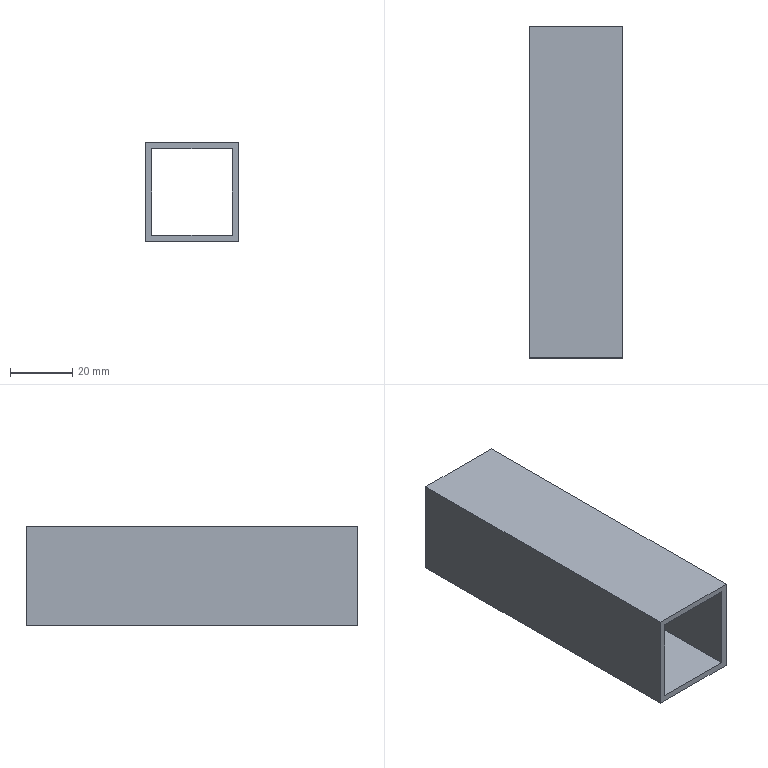Part | NX | features solid 2 | 1 solid | 10 faces | box 30 x 107 x 32 mm | volume 24824 mm3 | plane 10
STEP:
#1=CARTESIAN_POINT('',(475.,468.,-63.));
#2=VERTEX_POINT('',#1);
#3=CARTESIAN_POINT('',(445.,468.,-63.));
#4=VERTEX_POINT('',#3);
#5=CARTESIAN_POINT('',(475.,468.,-63.));
#6=DIRECTION('',(-1.,0.,0.));
#7=VECTOR('',#6,1000.);
#8=LINE('',#5,#7);
#9=EDGE_CURVE('',#2,#4,#8,.T.);
#10=ORIENTED_EDGE('',*,*,#9,.T.);
#11=CARTESIAN_POINT('',(445.,468.,-95.));
#12=VERTEX_POINT('',#11);
#13=CARTESIAN_POINT('',(445.,468.,-90.));
#14=DIRECTION('',(0.,0.,-1.));
#15=VECTOR('',#14,1000.);
#16=LINE('',#13,#15);
#17=EDGE_CURVE('',#4,#12,#16,.T.);
#18=ORIENTED_EDGE('',*,*,#17,.T.);
#19=CARTESIAN_POINT('',(475.,468.,-95.));
#20=VERTEX_POINT('',#19);
#21=CARTESIAN_POINT('',(445.,468.,-95.));
#22=DIRECTION('',(1.,0.,0.));
#23=VECTOR('',#22,1000.);
#24=LINE('',#21,#23);
#25=EDGE_CURVE('',#20,#12,#24,.F.);
#26=ORIENTED_EDGE('',*,*,#25,.F.);
#27=CARTESIAN_POINT('',(475.,468.,-90.));
#28=DIRECTION('',(0.,0.,-1.));
#29=VECTOR('',#28,1000.);
#30=LINE('',#27,#29);
#31=EDGE_CURVE('',#2,#20,#30,.T.);
#32=ORIENTED_EDGE('',*,*,#31,.F.);
#33=EDGE_LOOP('',(#10,#18,#26,#32));
#34=FACE_BOUND('',#33,.T.);
#35=CARTESIAN_POINT('',(473.,468.,-65.));
#36=VERTEX_POINT('',#35);
#37=CARTESIAN_POINT('',(447.,468.,-65.));
#38=VERTEX_POINT('',#37);
#39=CARTESIAN_POINT('',(475.,468.,-65.));
#40=DIRECTION('',(-1.,0.,0.));
#41=VECTOR('',#40,1000.);
#42=LINE('',#39,#41);
#43=EDGE_CURVE('',#36,#38,#42,.T.);
#44=ORIENTED_EDGE('',*,*,#43,.F.);
#45=CARTESIAN_POINT('',(473.,468.,-93.));
#46=VERTEX_POINT('',#45);
#47=CARTESIAN_POINT('',(473.,468.,-90.));
#48=DIRECTION('',(0.,0.,-1.));
#49=VECTOR('',#48,1000.);
#50=LINE('',#47,#49);
#51=EDGE_CURVE('',#36,#46,#50,.T.);
#52=ORIENTED_EDGE('',*,*,#51,.T.);
#53=CARTESIAN_POINT('',(447.,468.,-93.));
#54=VERTEX_POINT('',#53);
#55=CARTESIAN_POINT('',(445.,468.,-93.));
#56=DIRECTION('',(1.,0.,0.));
#57=VECTOR('',#56,1000.);
#58=LINE('',#55,#57);
#59=EDGE_CURVE('',#46,#54,#58,.F.);
#60=ORIENTED_EDGE('',*,*,#59,.T.);
#61=CARTESIAN_POINT('',(447.,468.,-90.));
#62=DIRECTION('',(0.,0.,-1.));
#63=VECTOR('',#62,1000.);
#64=LINE('',#61,#63);
#65=EDGE_CURVE('',#38,#54,#64,.T.);
#66=ORIENTED_EDGE('',*,*,#65,.F.);
#67=EDGE_LOOP('',(#44,#52,#60,#66));
#68=FACE_BOUND('',#67,.T.);
#69=CARTESIAN_POINT('',(475.,468.,-90.));
#70=DIRECTION('',(0.,1.,0.));
#71=DIRECTION('',(0.,0.,1.));
#72=AXIS2_PLACEMENT_3D('',#69,#70,#71);
#73=PLANE('',#72);
#74=ADVANCED_FACE('',(#34,#68),#73,.F.);
#75=CARTESIAN_POINT('',(475.,575.,-95.));
#76=VERTEX_POINT('',#75);
#77=CARTESIAN_POINT('',(445.,575.,-95.));
#78=VERTEX_POINT('',#77);
#79=CARTESIAN_POINT('',(672.,575.,-95.));
#80=DIRECTION('',(-1.,0.,0.));
#81=VECTOR('',#80,1000.);
#82=LINE('',#79,#81);
#83=EDGE_CURVE('',#76,#78,#82,.T.);
#84=ORIENTED_EDGE('',*,*,#83,.T.);
#85=CARTESIAN_POINT('',(445.,575.,-63.));
#86=VERTEX_POINT('',#85);
#87=CARTESIAN_POINT('',(445.,575.,-63.));
#88=DIRECTION('',(0.,0.,1.));
#89=VECTOR('',#88,1000.);
#90=LINE('',#87,#89);
#91=EDGE_CURVE('',#86,#78,#90,.F.);
#92=ORIENTED_EDGE('',*,*,#91,.F.);
#93=CARTESIAN_POINT('',(475.,575.,-63.));
#94=VERTEX_POINT('',#93);
#95=CARTESIAN_POINT('',(445.,575.,-63.));
#96=DIRECTION('',(1.,0.,0.));
#97=VECTOR('',#96,1000.);
#98=LINE('',#95,#97);
#99=EDGE_CURVE('',#94,#86,#98,.F.);
#100=ORIENTED_EDGE('',*,*,#99,.F.);
#101=CARTESIAN_POINT('',(475.,575.,-63.));
#102=DIRECTION('',(0.,0.,1.));
#103=VECTOR('',#102,1000.);
#104=LINE('',#101,#103);
#105=EDGE_CURVE('',#94,#76,#104,.F.);
#106=ORIENTED_EDGE('',*,*,#105,.T.);
#107=EDGE_LOOP('',(#84,#92,#100,#106));
#108=FACE_BOUND('',#107,.T.);
#109=CARTESIAN_POINT('',(473.,575.,-93.));
#110=VERTEX_POINT('',#109);
#111=CARTESIAN_POINT('',(447.,575.,-93.));
#112=VERTEX_POINT('',#111);
#113=CARTESIAN_POINT('',(672.,575.,-93.));
#114=DIRECTION('',(-1.,0.,0.));
#115=VECTOR('',#114,1000.);
#116=LINE('',#113,#115);
#117=EDGE_CURVE('',#110,#112,#116,.T.);
#118=ORIENTED_EDGE('',*,*,#117,.F.);
#119=CARTESIAN_POINT('',(473.,575.,-65.));
#120=VERTEX_POINT('',#119);
#121=CARTESIAN_POINT('',(473.,575.,-63.));
#122=DIRECTION('',(0.,0.,1.));
#123=VECTOR('',#122,1000.);
#124=LINE('',#121,#123);
#125=EDGE_CURVE('',#120,#110,#124,.F.);
#126=ORIENTED_EDGE('',*,*,#125,.F.);
#127=CARTESIAN_POINT('',(447.,575.,-65.));
#128=VERTEX_POINT('',#127);
#129=CARTESIAN_POINT('',(445.,575.,-65.));
#130=DIRECTION('',(1.,0.,0.));
#131=VECTOR('',#130,1000.);
#132=LINE('',#129,#131);
#133=EDGE_CURVE('',#120,#128,#132,.F.);
#134=ORIENTED_EDGE('',*,*,#133,.T.);
#135=CARTESIAN_POINT('',(447.,575.,-63.));
#136=DIRECTION('',(0.,0.,1.));
#137=VECTOR('',#136,1000.);
#138=LINE('',#135,#137);
#139=EDGE_CURVE('',#128,#112,#138,.F.);
#140=ORIENTED_EDGE('',*,*,#139,.T.);
#141=EDGE_LOOP('',(#118,#126,#134,#140));
#142=FACE_BOUND('',#141,.T.);
#143=CARTESIAN_POINT('',(672.,575.,-63.));
#144=DIRECTION('',(0.,1.,0.));
#145=DIRECTION('',(0.,0.,1.));
#146=AXIS2_PLACEMENT_3D('',#143,#144,#145);
#147=PLANE('',#146);
#148=ADVANCED_FACE('',(#108,#142),#147,.T.);
#149=ORIENTED_EDGE('',*,*,#25,.T.);
#150=CARTESIAN_POINT('',(445.,378.,-95.));
#151=DIRECTION('',(0.,1.,0.));
#152=VECTOR('',#151,1000.);
#153=LINE('',#150,#152);
#154=EDGE_CURVE('',#12,#78,#153,.T.);
#155=ORIENTED_EDGE('',*,*,#154,.T.);
#156=ORIENTED_EDGE('',*,*,#83,.F.);
#157=CARTESIAN_POINT('',(475.,378.,-95.));
#158=DIRECTION('',(0.,-1.,0.));
#159=VECTOR('',#158,1000.);
#160=LINE('',#157,#159);
#161=EDGE_CURVE('',#20,#76,#160,.F.);
#162=ORIENTED_EDGE('',*,*,#161,.F.);
#163=EDGE_LOOP('',(#149,#155,#156,#162));
#164=FACE_BOUND('',#163,.T.);
#165=CARTESIAN_POINT('',(445.,378.,-95.));
#166=DIRECTION('',(0.,0.,-1.));
#167=DIRECTION('',(0.,1.,0.));
#168=AXIS2_PLACEMENT_3D('',#165,#166,#167);
#169=PLANE('',#168);
#170=ADVANCED_FACE('',(#164),#169,.T.);
#171=CARTESIAN_POINT('',(475.,378.,-63.));
#172=DIRECTION('',(0.,1.,0.));
#173=VECTOR('',#172,1000.);
#174=LINE('',#171,#173);
#175=EDGE_CURVE('',#2,#94,#174,.T.);
#176=ORIENTED_EDGE('',*,*,#175,.T.);
#177=ORIENTED_EDGE('',*,*,#99,.T.);
#178=CARTESIAN_POINT('',(445.,378.,-63.));
#179=DIRECTION('',(0.,1.,0.));
#180=VECTOR('',#179,1000.);
#181=LINE('',#178,#180);
#182=EDGE_CURVE('',#4,#86,#181,.T.);
#183=ORIENTED_EDGE('',*,*,#182,.F.);
#184=ORIENTED_EDGE('',*,*,#9,.F.);
#185=EDGE_LOOP('',(#176,#177,#183,#184));
#186=FACE_BOUND('',#185,.T.);
#187=CARTESIAN_POINT('',(445.,378.,-63.));
#188=DIRECTION('',(0.,0.,-1.));
#189=DIRECTION('',(0.,1.,0.));
#190=AXIS2_PLACEMENT_3D('',#187,#188,#189);
#191=PLANE('',#190);
#192=ADVANCED_FACE('',(#186),#191,.F.);
#193=ORIENTED_EDGE('',*,*,#91,.T.);
#194=ORIENTED_EDGE('',*,*,#154,.F.);
#195=ORIENTED_EDGE('',*,*,#17,.F.);
#196=ORIENTED_EDGE('',*,*,#182,.T.);
#197=EDGE_LOOP('',(#193,#194,#195,#196));
#198=FACE_BOUND('',#197,.T.);
#199=CARTESIAN_POINT('',(445.,378.,-63.));
#200=DIRECTION('',(1.,0.,0.));
#201=DIRECTION('',(0.,0.,1.));
#202=AXIS2_PLACEMENT_3D('',#199,#200,#201);
#203=PLANE('',#202);
#204=ADVANCED_FACE('',(#198),#203,.F.);
#205=ORIENTED_EDGE('',*,*,#105,.F.);
#206=ORIENTED_EDGE('',*,*,#175,.F.);
#207=ORIENTED_EDGE('',*,*,#31,.T.);
#208=ORIENTED_EDGE('',*,*,#161,.T.);
#209=EDGE_LOOP('',(#205,#206,#207,#208));
#210=FACE_BOUND('',#209,.T.);
#211=CARTESIAN_POINT('',(475.,378.,-63.));
#212=DIRECTION('',(1.,0.,0.));
#213=DIRECTION('',(0.,0.,1.));
#214=AXIS2_PLACEMENT_3D('',#211,#212,#213);
#215=PLANE('',#214);
#216=ADVANCED_FACE('',(#210),#215,.T.);
#217=CARTESIAN_POINT('',(447.,378.,-93.));
#218=DIRECTION('',(0.,-1.,0.));
#219=VECTOR('',#218,1000.);
#220=LINE('',#217,#219);
#221=EDGE_CURVE('',#54,#112,#220,.F.);
#222=ORIENTED_EDGE('',*,*,#221,.F.);
#223=ORIENTED_EDGE('',*,*,#59,.F.);
#224=CARTESIAN_POINT('',(473.,378.,-93.));
#225=DIRECTION('',(0.,-1.,0.));
#226=VECTOR('',#225,1000.);
#227=LINE('',#224,#226);
#228=EDGE_CURVE('',#46,#110,#227,.F.);
#229=ORIENTED_EDGE('',*,*,#228,.T.);
#230=ORIENTED_EDGE('',*,*,#117,.T.);
#231=EDGE_LOOP('',(#222,#223,#229,#230));
#232=FACE_BOUND('',#231,.T.);
#233=CARTESIAN_POINT('',(445.,378.,-93.));
#234=DIRECTION('',(0.,0.,-1.));
#235=DIRECTION('',(0.,1.,0.));
#236=AXIS2_PLACEMENT_3D('',#233,#234,#235);
#237=PLANE('',#236);
#238=ADVANCED_FACE('',(#232),#237,.F.);
#239=CARTESIAN_POINT('',(473.,378.,-65.));
#240=DIRECTION('',(0.,1.,0.));
#241=VECTOR('',#240,1000.);
#242=LINE('',#239,#241);
#243=EDGE_CURVE('',#36,#120,#242,.T.);
#244=ORIENTED_EDGE('',*,*,#243,.F.);
#245=ORIENTED_EDGE('',*,*,#43,.T.);
#246=CARTESIAN_POINT('',(447.,378.,-65.));
#247=DIRECTION('',(0.,1.,0.));
#248=VECTOR('',#247,1000.);
#249=LINE('',#246,#248);
#250=EDGE_CURVE('',#38,#128,#249,.T.);
#251=ORIENTED_EDGE('',*,*,#250,.T.);
#252=ORIENTED_EDGE('',*,*,#133,.F.);
#253=EDGE_LOOP('',(#244,#245,#251,#252));
#254=FACE_BOUND('',#253,.T.);
#255=CARTESIAN_POINT('',(445.,378.,-65.));
#256=DIRECTION('',(0.,0.,-1.));
#257=DIRECTION('',(0.,1.,0.));
#258=AXIS2_PLACEMENT_3D('',#255,#256,#257);
#259=PLANE('',#258);
#260=ADVANCED_FACE('',(#254),#259,.T.);
#261=ORIENTED_EDGE('',*,*,#139,.F.);
#262=ORIENTED_EDGE('',*,*,#250,.F.);
#263=ORIENTED_EDGE('',*,*,#65,.T.);
#264=ORIENTED_EDGE('',*,*,#221,.T.);
#265=EDGE_LOOP('',(#261,#262,#263,#264));
#266=FACE_BOUND('',#265,.T.);
#267=CARTESIAN_POINT('',(447.,378.,-63.));
#268=DIRECTION('',(1.,0.,0.));
#269=DIRECTION('',(0.,0.,1.));
#270=AXIS2_PLACEMENT_3D('',#267,#268,#269);
#271=PLANE('',#270);
#272=ADVANCED_FACE('',(#266),#271,.T.);
#273=ORIENTED_EDGE('',*,*,#125,.T.);
#274=ORIENTED_EDGE('',*,*,#228,.F.);
#275=ORIENTED_EDGE('',*,*,#51,.F.);
#276=ORIENTED_EDGE('',*,*,#243,.T.);
#277=EDGE_LOOP('',(#273,#274,#275,#276));
#278=FACE_BOUND('',#277,.T.);
#279=CARTESIAN_POINT('',(473.,378.,-63.));
#280=DIRECTION('',(1.,0.,0.));
#281=DIRECTION('',(0.,0.,1.));
#282=AXIS2_PLACEMENT_3D('',#279,#280,#281);
#283=PLANE('',#282);
#284=ADVANCED_FACE('',(#278),#283,.F.);
#285=CLOSED_SHELL('',(#74,#148,#170,#192,#204,#216,#238,#260,#272,#284));
#286=MANIFOLD_SOLID_BREP('',#285);
#287=(LENGTH_UNIT()NAMED_UNIT(*)SI_UNIT(.MILLI.,.METRE.));
#288=UNCERTAINTY_MEASURE_WITH_UNIT(LENGTH_MEASURE(0.00001),#287,'','');
#289=(NAMED_UNIT(*)PLANE_ANGLE_UNIT()SI_UNIT($,.RADIAN.));
#290=(NAMED_UNIT(*)SI_UNIT($,.STERADIAN.)SOLID_ANGLE_UNIT());
#291=(GEOMETRIC_REPRESENTATION_CONTEXT(3)GLOBAL_UNCERTAINTY_ASSIGNED_CONTEXT((#288))GLOBAL_UNIT_ASSIGNED_CONTEXT((#287,#289,#290))REPRESENTATION_CONTEXT('',''));
#292=ADVANCED_BREP_SHAPE_REPRESENTATION('',(#286),#291);